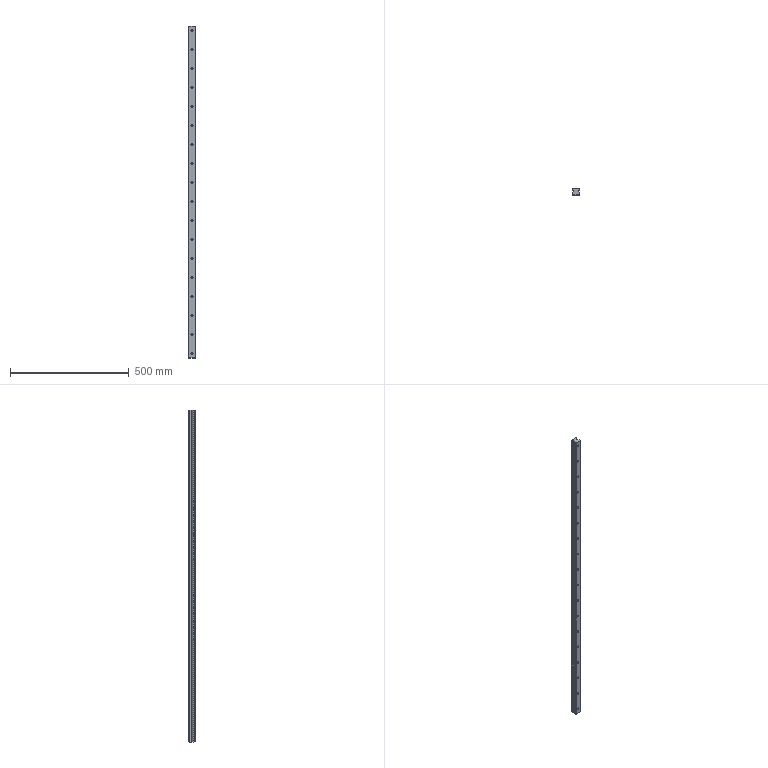Part | SolidWorks | features BaseBody 1 | 1 solid | 186 faces | box 28 x 26 x 1400 mm | volume 851786 mm3 | cylinder 106 | plane 80 | commonest cylinder face diameters 9 x36 14 x36 1.152 x10 1.613 x8 0.922 x5 1.373 x3